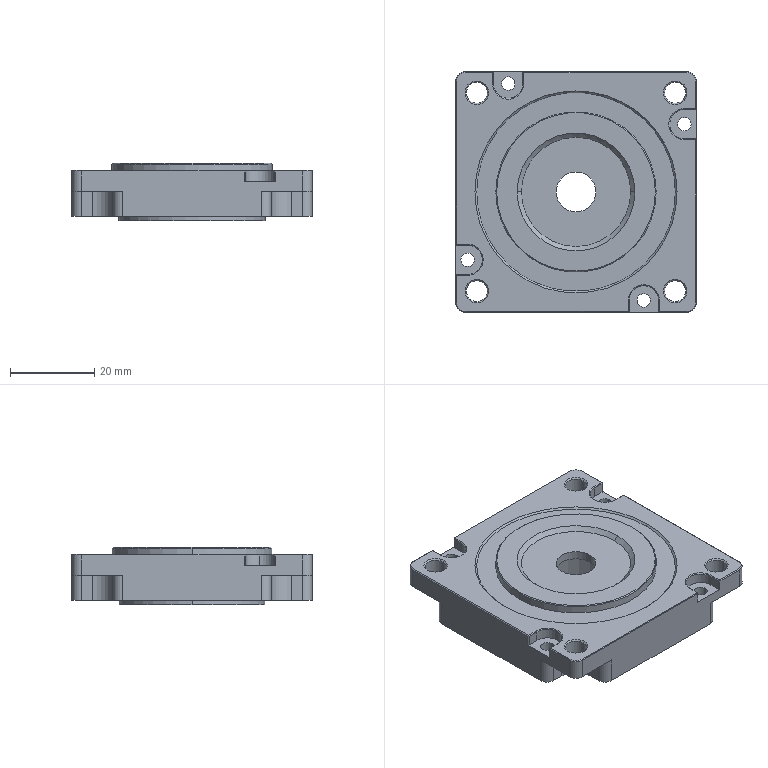Part | NX | features BREP 1 | 1 solid | 147 faces | box 57.15 x 57.15 x 13.6 mm | volume 19483 mm3 | plane 77 | cylinder 47 | cone 23 | commonest cylinder face diameters 4.6 x12 3.2 x8 5 x8 9.5 x6 7 x5 22 x2